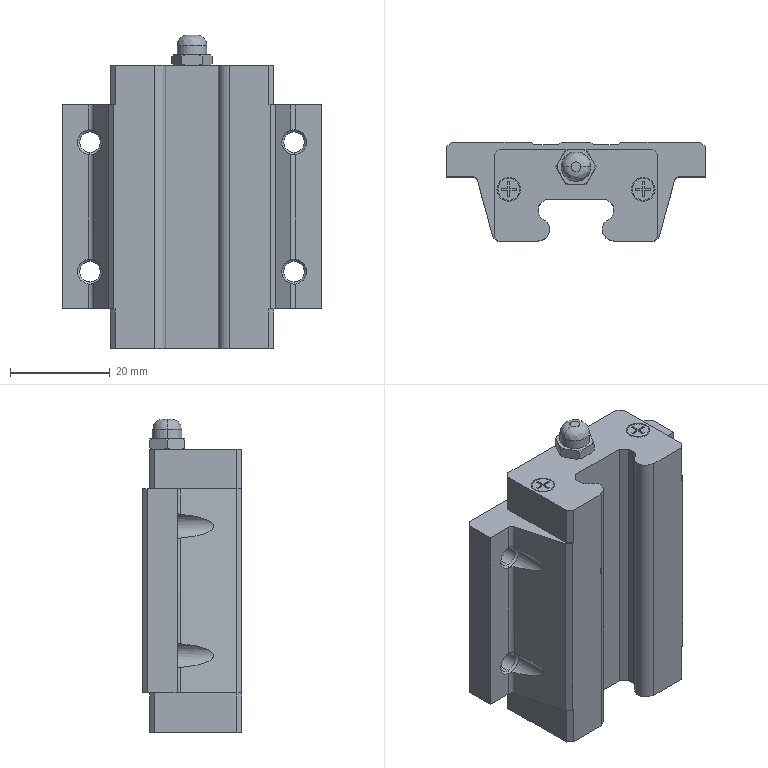Part | STEP file | 0245_Z_018_SX2WT24-1480_2 | 1 solid | 199 faces | box 52 x 20 x 63 mm | volume 37170 mm3 | plane 98 | cylinder 69 | cone 30 | spline 2 | commonest cylinder face diameters 3.08 x20 5 x12 4.4 x11 4.134 x8 4.8 x8 2 x6